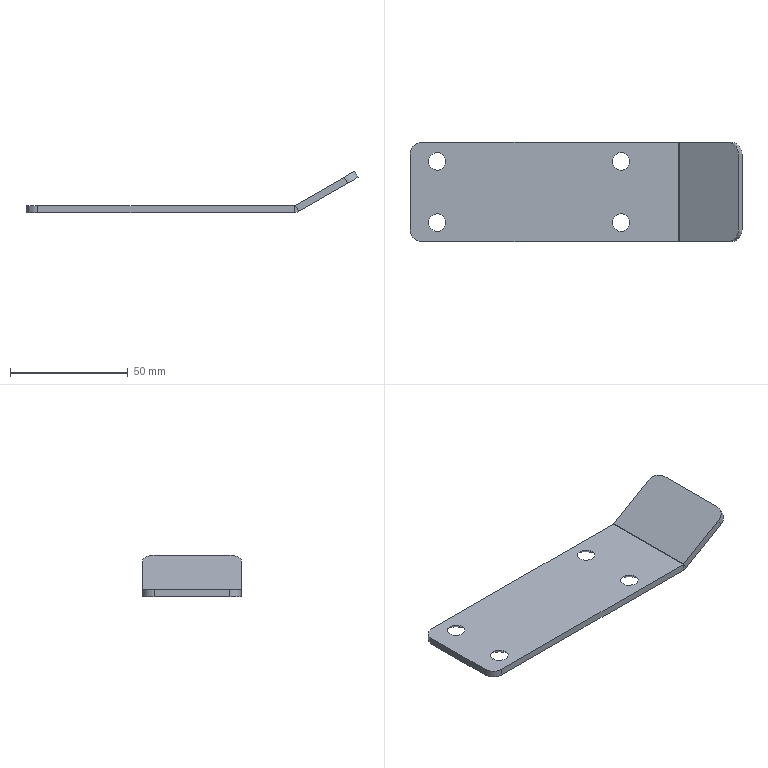Part | SolidWorks | features EdgeFlange 1, Fillet 1, FlatPattern 1, HoleWzd 1, SMBaseFlange 1, SheetMetal 1 | 1 solid | 26 faces | box 140.785 x 42 x 17.598 mm | volume 17021 mm3 | plane 12 | cone 8 | cylinder 6 | commonest cylinder face diameters 10 x4 1.473 x1 7.473 x1
STEP:
#1=CARTESIAN_POINT('',(-52.22,34.,0.));
#2=VERTEX_POINT('',#1);
#3=CARTESIAN_POINT('',(-44.78,34.,0.));
#4=VERTEX_POINT('',#3);
#5=CARTESIAN_POINT('',(-48.5,34.,0.));
#6=DIRECTION('',(0.,0.,1.));
#7=DIRECTION('',(1.,0.,0.));
#8=AXIS2_PLACEMENT_3D('',#5,#6,#7);
#9=CIRCLE('',#8,3.72);
#10=EDGE_CURVE('',#2,#4,#9,.T.);
#11=ORIENTED_EDGE('',*,*,#10,.T.);
#12=CARTESIAN_POINT('',(-41.78,34.,-3.));
#13=VERTEX_POINT('',#12);
#14=CARTESIAN_POINT('',(-41.78,34.,-3.));
#15=DIRECTION('',(0.7071,0.,-0.7071));
#16=VECTOR('',#15,1000.);
#17=LINE('',#14,#16);
#18=EDGE_CURVE('',#4,#13,#17,.T.);
#19=ORIENTED_EDGE('',*,*,#18,.T.);
#20=CARTESIAN_POINT('',(-55.22,34.,-3.));
#21=VERTEX_POINT('',#20);
#22=CARTESIAN_POINT('',(-48.5,34.,-3.));
#23=DIRECTION('',(0.,0.,-1.));
#24=DIRECTION('',(-1.,0.,0.));
#25=AXIS2_PLACEMENT_3D('',#22,#23,#24);
#26=CIRCLE('',#25,6.72);
#27=EDGE_CURVE('',#13,#21,#26,.T.);
#28=ORIENTED_EDGE('',*,*,#27,.T.);
#29=CARTESIAN_POINT('',(-55.22,34.,-3.));
#30=DIRECTION('',(-0.7071,0.,-0.7071));
#31=VECTOR('',#30,1000.);
#32=LINE('',#29,#31);
#33=EDGE_CURVE('',#2,#21,#32,.T.);
#34=ORIENTED_EDGE('',*,*,#33,.F.);
#35=EDGE_LOOP('',(#11,#19,#28,#34));
#36=FACE_OUTER_BOUND('',#35,.T.);
#37=CARTESIAN_POINT('',(-48.5,34.,-3.));
#38=DIRECTION('',(0.,0.,-1.));
#39=DIRECTION('',(-1.,0.,0.));
#40=AXIS2_PLACEMENT_3D('',#37,#38,#39);
#41=CONICAL_SURFACE('',#40,6.72,0.7854);
#42=ADVANCED_FACE('',(#36),#41,.F.);
#43=CARTESIAN_POINT('',(-52.22,8.,0.));
#44=VERTEX_POINT('',#43);
#45=CARTESIAN_POINT('',(-44.78,8.,0.));
#46=VERTEX_POINT('',#45);
#47=CARTESIAN_POINT('',(-48.5,8.,0.));
#48=DIRECTION('',(0.,0.,1.));
#49=DIRECTION('',(1.,0.,0.));
#50=AXIS2_PLACEMENT_3D('',#47,#48,#49);
#51=CIRCLE('',#50,3.72);
#52=EDGE_CURVE('',#44,#46,#51,.T.);
#53=ORIENTED_EDGE('',*,*,#52,.T.);
#54=CARTESIAN_POINT('',(-41.78,8.,-3.));
#55=VERTEX_POINT('',#54);
#56=CARTESIAN_POINT('',(-41.78,8.,-3.));
#57=DIRECTION('',(0.7071,0.,-0.7071));
#58=VECTOR('',#57,1000.);
#59=LINE('',#56,#58);
#60=EDGE_CURVE('',#46,#55,#59,.T.);
#61=ORIENTED_EDGE('',*,*,#60,.T.);
#62=CARTESIAN_POINT('',(-55.22,8.,-3.));
#63=VERTEX_POINT('',#62);
#64=CARTESIAN_POINT('',(-48.5,8.,-3.));
#65=DIRECTION('',(0.,0.,-1.));
#66=DIRECTION('',(-1.,0.,0.));
#67=AXIS2_PLACEMENT_3D('',#64,#65,#66);
#68=CIRCLE('',#67,6.72);
#69=EDGE_CURVE('',#55,#63,#68,.T.);
#70=ORIENTED_EDGE('',*,*,#69,.T.);
#71=CARTESIAN_POINT('',(-55.22,8.,-3.));
#72=DIRECTION('',(-0.7071,0.,-0.7071));
#73=VECTOR('',#72,1000.);
#74=LINE('',#71,#73);
#75=EDGE_CURVE('',#44,#63,#74,.T.);
#76=ORIENTED_EDGE('',*,*,#75,.F.);
#77=EDGE_LOOP('',(#53,#61,#70,#76));
#78=FACE_OUTER_BOUND('',#77,.T.);
#79=CARTESIAN_POINT('',(-48.5,8.,-3.));
#80=DIRECTION('',(0.,0.,-1.));
#81=DIRECTION('',(-1.,0.,0.));
#82=AXIS2_PLACEMENT_3D('',#79,#80,#81);
#83=CONICAL_SURFACE('',#82,6.72,0.7854);
#84=ADVANCED_FACE('',(#78),#83,.F.);
#85=CARTESIAN_POINT('',(25.78,34.,0.));
#86=VERTEX_POINT('',#85);
#87=CARTESIAN_POINT('',(33.22,34.,0.));
#88=VERTEX_POINT('',#87);
#89=CARTESIAN_POINT('',(29.5,34.,0.));
#90=DIRECTION('',(0.,0.,1.));
#91=DIRECTION('',(1.,0.,0.));
#92=AXIS2_PLACEMENT_3D('',#89,#90,#91);
#93=CIRCLE('',#92,3.72);
#94=EDGE_CURVE('',#86,#88,#93,.T.);
#95=ORIENTED_EDGE('',*,*,#94,.T.);
#96=CARTESIAN_POINT('',(36.22,34.,-3.));
#97=VERTEX_POINT('',#96);
#98=CARTESIAN_POINT('',(36.22,34.,-3.));
#99=DIRECTION('',(0.7071,0.,-0.7071));
#100=VECTOR('',#99,1000.);
#101=LINE('',#98,#100);
#102=EDGE_CURVE('',#88,#97,#101,.T.);
#103=ORIENTED_EDGE('',*,*,#102,.T.);
#104=CARTESIAN_POINT('',(22.78,34.,-3.));
#105=VERTEX_POINT('',#104);
#106=CARTESIAN_POINT('',(29.5,34.,-3.));
#107=DIRECTION('',(0.,0.,-1.));
#108=DIRECTION('',(-1.,0.,0.));
#109=AXIS2_PLACEMENT_3D('',#106,#107,#108);
#110=CIRCLE('',#109,6.72);
#111=EDGE_CURVE('',#97,#105,#110,.T.);
#112=ORIENTED_EDGE('',*,*,#111,.T.);
#113=CARTESIAN_POINT('',(22.78,34.,-3.));
#114=DIRECTION('',(-0.7071,0.,-0.7071));
#115=VECTOR('',#114,1000.);
#116=LINE('',#113,#115);
#117=EDGE_CURVE('',#86,#105,#116,.T.);
#118=ORIENTED_EDGE('',*,*,#117,.F.);
#119=EDGE_LOOP('',(#95,#103,#112,#118));
#120=FACE_OUTER_BOUND('',#119,.T.);
#121=CARTESIAN_POINT('',(29.5,34.,-3.));
#122=DIRECTION('',(0.,0.,-1.));
#123=DIRECTION('',(-1.,0.,0.));
#124=AXIS2_PLACEMENT_3D('',#121,#122,#123);
#125=CONICAL_SURFACE('',#124,6.72,0.7854);
#126=ADVANCED_FACE('',(#120),#125,.F.);
#127=CARTESIAN_POINT('',(25.78,8.,0.));
#128=VERTEX_POINT('',#127);
#129=CARTESIAN_POINT('',(33.22,8.,0.));
#130=VERTEX_POINT('',#129);
#131=CARTESIAN_POINT('',(29.5,8.,0.));
#132=DIRECTION('',(0.,0.,1.));
#133=DIRECTION('',(1.,0.,0.));
#134=AXIS2_PLACEMENT_3D('',#131,#132,#133);
#135=CIRCLE('',#134,3.72);
#136=EDGE_CURVE('',#128,#130,#135,.T.);
#137=ORIENTED_EDGE('',*,*,#136,.T.);
#138=CARTESIAN_POINT('',(36.22,8.,-3.));
#139=VERTEX_POINT('',#138);
#140=CARTESIAN_POINT('',(36.22,8.,-3.));
#141=DIRECTION('',(0.7071,0.,-0.7071));
#142=VECTOR('',#141,1000.);
#143=LINE('',#140,#142);
#144=EDGE_CURVE('',#130,#139,#143,.T.);
#145=ORIENTED_EDGE('',*,*,#144,.T.);
#146=CARTESIAN_POINT('',(22.78,8.,-3.));
#147=VERTEX_POINT('',#146);
#148=CARTESIAN_POINT('',(29.5,8.,-3.));
#149=DIRECTION('',(0.,0.,-1.));
#150=DIRECTION('',(-1.,0.,0.));
#151=AXIS2_PLACEMENT_3D('',#148,#149,#150);
#152=CIRCLE('',#151,6.72);
#153=EDGE_CURVE('',#139,#147,#152,.T.);
#154=ORIENTED_EDGE('',*,*,#153,.T.);
#155=CARTESIAN_POINT('',(22.78,8.,-3.));
#156=DIRECTION('',(-0.7071,0.,-0.7071));
#157=VECTOR('',#156,1000.);
#158=LINE('',#155,#157);
#159=EDGE_CURVE('',#128,#147,#158,.T.);
#160=ORIENTED_EDGE('',*,*,#159,.F.);
#161=EDGE_LOOP('',(#137,#145,#154,#160));
#162=FACE_OUTER_BOUND('',#161,.T.);
#163=CARTESIAN_POINT('',(29.5,8.,-3.));
#164=DIRECTION('',(0.,0.,-1.));
#165=DIRECTION('',(-1.,0.,0.));
#166=AXIS2_PLACEMENT_3D('',#163,#164,#165);
#167=CONICAL_SURFACE('',#166,6.72,0.7854);
#168=ADVANCED_FACE('',(#162),#167,.F.);
#169=CARTESIAN_POINT('',(53.803,42.,-3.));
#170=VERTEX_POINT('',#169);
#171=CARTESIAN_POINT('',(-55.,42.,-3.));
#172=VERTEX_POINT('',#171);
#173=CARTESIAN_POINT('',(-60.,42.,-3.));
#174=DIRECTION('',(-1.,0.,0.));
#175=VECTOR('',#174,1000.);
#176=LINE('',#173,#175);
#177=EDGE_CURVE('',#170,#172,#176,.T.);
#178=ORIENTED_EDGE('',*,*,#177,.T.);
#179=CARTESIAN_POINT('',(-55.,42.,0.));
#180=VERTEX_POINT('',#179);
#181=CARTESIAN_POINT('',(-55.,42.,-3.));
#182=DIRECTION('',(0.,0.,1.));
#183=VECTOR('',#182,1000.);
#184=LINE('',#181,#183);
#185=EDGE_CURVE('',#172,#180,#184,.T.);
#186=ORIENTED_EDGE('',*,*,#185,.T.);
#187=CARTESIAN_POINT('',(53.803,42.,0.));
#188=VERTEX_POINT('',#187);
#189=CARTESIAN_POINT('',(-60.,42.,0.));
#190=DIRECTION('',(-1.,0.,0.));
#191=VECTOR('',#190,1000.);
#192=LINE('',#189,#191);
#193=EDGE_CURVE('',#188,#180,#192,.T.);
#194=ORIENTED_EDGE('',*,*,#193,.F.);
#195=CARTESIAN_POINT('',(53.803,42.,0.));
#196=DIRECTION('',(0.,0.,-1.));
#197=VECTOR('',#196,1000.);
#198=LINE('',#195,#197);
#199=EDGE_CURVE('',#188,#170,#198,.T.);
#200=ORIENTED_EDGE('',*,*,#199,.T.);
#201=EDGE_LOOP('',(#178,#186,#194,#200));
#202=FACE_OUTER_BOUND('',#201,.T.);
#203=CARTESIAN_POINT('',(-60.,42.,-3.));
#204=DIRECTION('',(0.,1.,0.));
#205=DIRECTION('',(0.,0.,1.));
#206=AXIS2_PLACEMENT_3D('',#203,#204,#205);
#207=PLANE('',#206);
#208=ADVANCED_FACE('',(#202),#207,.T.);
#209=CARTESIAN_POINT('',(-48.5,34.,-3.));
#210=DIRECTION('',(0.,0.,-1.));
#211=DIRECTION('',(-1.,0.,0.));
#212=AXIS2_PLACEMENT_3D('',#209,#210,#211);
#213=CIRCLE('',#212,6.72);
#214=EDGE_CURVE('',#21,#13,#213,.T.);
#215=ORIENTED_EDGE('',*,*,#214,.F.);
#216=ORIENTED_EDGE('',*,*,#27,.F.);
#217=EDGE_LOOP('',(#215,#216));
#218=FACE_BOUND('',#217,.T.);
#219=CARTESIAN_POINT('',(-48.5,8.,-3.));
#220=DIRECTION('',(0.,0.,-1.));
#221=DIRECTION('',(-1.,0.,0.));
#222=AXIS2_PLACEMENT_3D('',#219,#220,#221);
#223=CIRCLE('',#222,6.72);
#224=EDGE_CURVE('',#63,#55,#223,.T.);
#225=ORIENTED_EDGE('',*,*,#224,.F.);
#226=ORIENTED_EDGE('',*,*,#69,.F.);
#227=EDGE_LOOP('',(#225,#226));
#228=FACE_BOUND('',#227,.T.);
#229=CARTESIAN_POINT('',(29.5,34.,-3.));
#230=DIRECTION('',(0.,0.,-1.));
#231=DIRECTION('',(-1.,0.,0.));
#232=AXIS2_PLACEMENT_3D('',#229,#230,#231);
#233=CIRCLE('',#232,6.72);
#234=EDGE_CURVE('',#105,#97,#233,.T.);
#235=ORIENTED_EDGE('',*,*,#234,.F.);
#236=ORIENTED_EDGE('',*,*,#111,.F.);
#237=EDGE_LOOP('',(#235,#236));
#238=FACE_BOUND('',#237,.T.);
#239=CARTESIAN_POINT('',(29.5,8.,-3.));
#240=DIRECTION('',(0.,0.,-1.));
#241=DIRECTION('',(-1.,0.,0.));
#242=AXIS2_PLACEMENT_3D('',#239,#240,#241);
#243=CIRCLE('',#242,6.72);
#244=EDGE_CURVE('',#147,#139,#243,.T.);
#245=ORIENTED_EDGE('',*,*,#244,.F.);
#246=ORIENTED_EDGE('',*,*,#153,.F.);
#247=EDGE_LOOP('',(#245,#246));
#248=FACE_BOUND('',#247,.T.);
#249=CARTESIAN_POINT('',(-55.,0.,-3.));
#250=VERTEX_POINT('',#249);
#251=CARTESIAN_POINT('',(53.803,0.,-3.));
#252=VERTEX_POINT('',#251);
#253=CARTESIAN_POINT('',(-60.,0.,-3.));
#254=DIRECTION('',(1.,0.,0.));
#255=VECTOR('',#254,1000.);
#256=LINE('',#253,#255);
#257=EDGE_CURVE('',#250,#252,#256,.T.);
#258=ORIENTED_EDGE('',*,*,#257,.F.);
#259=CARTESIAN_POINT('',(-60.,5.,-3.));
#260=VERTEX_POINT('',#259);
#261=CARTESIAN_POINT('',(-55.,5.,-3.));
#262=DIRECTION('',(0.,0.,-1.));
#263=DIRECTION('',(1.,0.,0.));
#264=AXIS2_PLACEMENT_3D('',#261,#262,#263);
#265=CIRCLE('',#264,5.);
#266=EDGE_CURVE('',#250,#260,#265,.T.);
#267=ORIENTED_EDGE('',*,*,#266,.T.);
#268=CARTESIAN_POINT('',(-60.,37.,-3.));
#269=VERTEX_POINT('',#268);
#270=CARTESIAN_POINT('',(-60.,42.,-3.));
#271=DIRECTION('',(0.,-1.,0.));
#272=VECTOR('',#271,1000.);
#273=LINE('',#270,#272);
#274=EDGE_CURVE('',#269,#260,#273,.T.);
#275=ORIENTED_EDGE('',*,*,#274,.F.);
#276=CARTESIAN_POINT('',(-55.,37.,-3.));
#277=DIRECTION('',(0.,0.,-1.));
#278=DIRECTION('',(1.,0.,0.));
#279=AXIS2_PLACEMENT_3D('',#276,#277,#278);
#280=CIRCLE('',#279,5.);
#281=EDGE_CURVE('',#269,#172,#280,.T.);
#282=ORIENTED_EDGE('',*,*,#281,.T.);
#283=ORIENTED_EDGE('',*,*,#177,.F.);
#284=CARTESIAN_POINT('',(53.803,42.,-3.));
#285=DIRECTION('',(0.,-1.,0.));
#286=VECTOR('',#285,1000.);
#287=LINE('',#284,#286);
#288=EDGE_CURVE('',#170,#252,#287,.T.);
#289=ORIENTED_EDGE('',*,*,#288,.T.);
#290=EDGE_LOOP('',(#258,#267,#275,#282,#283,#289));
#291=FACE_OUTER_BOUND('',#290,.T.);
#292=CARTESIAN_POINT('',(0.,0.,-3.));
#293=DIRECTION('',(0.,0.,1.));
#294=DIRECTION('',(1.,0.,0.));
#295=AXIS2_PLACEMENT_3D('',#292,#293,#294);
#296=PLANE('',#295);
#297=ADVANCED_FACE('',(#218,#228,#238,#248,#291),#296,.F.);
#298=ORIENTED_EDGE('',*,*,#10,.F.);
#299=CARTESIAN_POINT('',(-48.5,34.,0.));
#300=DIRECTION('',(0.,0.,1.));
#301=DIRECTION('',(1.,0.,0.));
#302=AXIS2_PLACEMENT_3D('',#299,#300,#301);
#303=CIRCLE('',#302,3.72);
#304=EDGE_CURVE('',#4,#2,#303,.T.);
#305=ORIENTED_EDGE('',*,*,#304,.F.);
#306=EDGE_LOOP('',(#298,#305));
#307=FACE_BOUND('',#306,.T.);
#308=ORIENTED_EDGE('',*,*,#52,.F.);
#309=CARTESIAN_POINT('',(-48.5,8.,0.));
#310=DIRECTION('',(0.,0.,1.));
#311=DIRECTION('',(1.,0.,0.));
#312=AXIS2_PLACEMENT_3D('',#309,#310,#311);
#313=CIRCLE('',#312,3.72);
#314=EDGE_CURVE('',#46,#44,#313,.T.);
#315=ORIENTED_EDGE('',*,*,#314,.F.);
#316=EDGE_LOOP('',(#308,#315));
#317=FACE_BOUND('',#316,.T.);
#318=ORIENTED_EDGE('',*,*,#94,.F.);
#319=CARTESIAN_POINT('',(29.5,34.,0.));
#320=DIRECTION('',(0.,0.,1.));
#321=DIRECTION('',(1.,0.,0.));
#322=AXIS2_PLACEMENT_3D('',#319,#320,#321);
#323=CIRCLE('',#322,3.72);
#324=EDGE_CURVE('',#88,#86,#323,.T.);
#325=ORIENTED_EDGE('',*,*,#324,.F.);
#326=EDGE_LOOP('',(#318,#325));
#327=FACE_BOUND('',#326,.T.);
#328=ORIENTED_EDGE('',*,*,#136,.F.);
#329=CARTESIAN_POINT('',(29.5,8.,0.));
#330=DIRECTION('',(0.,0.,1.));
#331=DIRECTION('',(1.,0.,0.));
#332=AXIS2_PLACEMENT_3D('',#329,#330,#331);
#333=CIRCLE('',#332,3.72);
#334=EDGE_CURVE('',#130,#128,#333,.T.);
#335=ORIENTED_EDGE('',*,*,#334,.F.);
#336=EDGE_LOOP('',(#328,#335));
#337=FACE_BOUND('',#336,.T.);
#338=CARTESIAN_POINT('',(-60.,37.,0.));
#339=VERTEX_POINT('',#338);
#340=CARTESIAN_POINT('',(-60.,5.,0.));
#341=VERTEX_POINT('',#340);
#342=CARTESIAN_POINT('',(-60.,42.,0.));
#343=DIRECTION('',(0.,-1.,0.));
#344=VECTOR('',#343,1000.);
#345=LINE('',#342,#344);
#346=EDGE_CURVE('',#339,#341,#345,.T.);
#347=ORIENTED_EDGE('',*,*,#346,.T.);
#348=CARTESIAN_POINT('',(-55.,0.,0.));
#349=VERTEX_POINT('',#348);
#350=CARTESIAN_POINT('',(-55.,5.,0.));
#351=DIRECTION('',(0.,0.,1.));
#352=DIRECTION('',(1.,0.,0.));
#353=AXIS2_PLACEMENT_3D('',#350,#351,#352);
#354=CIRCLE('',#353,5.);
#355=EDGE_CURVE('',#341,#349,#354,.T.);
#356=ORIENTED_EDGE('',*,*,#355,.T.);
#357=CARTESIAN_POINT('',(53.803,0.,0.));
#358=VERTEX_POINT('',#357);
#359=CARTESIAN_POINT('',(-60.,0.,0.));
#360=DIRECTION('',(1.,0.,0.));
#361=VECTOR('',#360,1000.);
#362=LINE('',#359,#361);
#363=EDGE_CURVE('',#349,#358,#362,.T.);
#364=ORIENTED_EDGE('',*,*,#363,.T.);
#365=CARTESIAN_POINT('',(53.803,42.,0.));
#366=DIRECTION('',(0.,-1.,0.));
#367=VECTOR('',#366,1000.);
#368=LINE('',#365,#367);
#369=EDGE_CURVE('',#188,#358,#368,.T.);
#370=ORIENTED_EDGE('',*,*,#369,.F.);
#371=ORIENTED_EDGE('',*,*,#193,.T.);
#372=CARTESIAN_POINT('',(-55.,37.,0.));
#373=DIRECTION('',(0.,0.,1.));
#374=DIRECTION('',(1.,0.,0.));
#375=AXIS2_PLACEMENT_3D('',#372,#373,#374);
#376=CIRCLE('',#375,5.);
#377=EDGE_CURVE('',#180,#339,#376,.T.);
#378=ORIENTED_EDGE('',*,*,#377,.T.);
#379=EDGE_LOOP('',(#347,#356,#364,#370,#371,#378));
#380=FACE_OUTER_BOUND('',#379,.T.);
#381=CARTESIAN_POINT('',(0.,0.,0.));
#382=DIRECTION('',(0.,0.,1.));
#383=DIRECTION('',(1.,0.,0.));
#384=AXIS2_PLACEMENT_3D('',#381,#382,#383);
#385=PLANE('',#384);
#386=ADVANCED_FACE('',(#307,#317,#327,#337,#380),#385,.T.);
#387=ORIENTED_EDGE('',*,*,#274,.T.);
#388=CARTESIAN_POINT('',(-60.,5.,-3.));
#389=DIRECTION('',(0.,0.,1.));
#390=VECTOR('',#389,1000.);
#391=LINE('',#388,#390);
#392=EDGE_CURVE('',#260,#341,#391,.T.);
#393=ORIENTED_EDGE('',*,*,#392,.T.);
#394=ORIENTED_EDGE('',*,*,#346,.F.);
#395=CARTESIAN_POINT('',(-60.,37.,-3.));
#396=DIRECTION('',(0.,0.,-1.));
#397=VECTOR('',#396,1000.);
#398=LINE('',#395,#397);
#399=EDGE_CURVE('',#339,#269,#398,.T.);
#400=ORIENTED_EDGE('',*,*,#399,.T.);
#401=EDGE_LOOP('',(#387,#393,#394,#400));
#402=FACE_OUTER_BOUND('',#401,.T.);
#403=CARTESIAN_POINT('',(-60.,42.,-3.));
#404=DIRECTION('',(-1.,0.,0.));
#405=DIRECTION('',(0.,0.,1.));
#406=AXIS2_PLACEMENT_3D('',#403,#404,#405);
#407=PLANE('',#406);
#408=ADVANCED_FACE('',(#402),#407,.T.);
#409=ORIENTED_EDGE('',*,*,#363,.F.);
#410=CARTESIAN_POINT('',(-55.,0.,-3.));
#411=DIRECTION('',(0.,0.,-1.));
#412=VECTOR('',#411,1000.);
#413=LINE('',#410,#412);
#414=EDGE_CURVE('',#349,#250,#413,.T.);
#415=ORIENTED_EDGE('',*,*,#414,.T.);
#416=ORIENTED_EDGE('',*,*,#257,.T.);
#417=CARTESIAN_POINT('',(53.803,0.,0.));
#418=DIRECTION('',(0.,0.,-1.));
#419=VECTOR('',#418,1000.);
#420=LINE('',#417,#419);
#421=EDGE_CURVE('',#358,#252,#420,.T.);
#422=ORIENTED_EDGE('',*,*,#421,.F.);
#423=EDGE_LOOP('',(#409,#415,#416,#422));
#424=FACE_OUTER_BOUND('',#423,.T.);
#425=CARTESIAN_POINT('',(-60.,0.,-3.));
#426=DIRECTION('',(0.,-1.,0.));
#427=DIRECTION('',(0.,0.,-1.));
#428=AXIS2_PLACEMENT_3D('',#425,#426,#427);
#429=PLANE('',#428);
#430=ADVANCED_FACE('',(#424),#429,.T.);
#431=CARTESIAN_POINT('',(54.171,0.,0.09869));
#432=VERTEX_POINT('',#431);
#433=CARTESIAN_POINT('',(55.671,0.,-2.499));
#434=VERTEX_POINT('',#433);
#435=CARTESIAN_POINT('',(55.671,0.,-2.499));
#436=DIRECTION('',(0.5,0.,-0.866));
#437=VECTOR('',#436,1000.);
#438=LINE('',#435,#437);
#439=EDGE_CURVE('',#432,#434,#438,.T.);
#440=ORIENTED_EDGE('',*,*,#439,.F.);
#441=CARTESIAN_POINT('',(53.803,0.,0.7366));
#442=DIRECTION('',(0.,-1.,0.));
#443=DIRECTION('',(0.,0.,1.));
#444=AXIS2_PLACEMENT_3D('',#441,#442,#443);
#445=CIRCLE('',#444,0.7366);
#446=EDGE_CURVE('',#358,#432,#445,.T.);
#447=ORIENTED_EDGE('',*,*,#446,.F.);
#448=ORIENTED_EDGE('',*,*,#421,.T.);
#449=CARTESIAN_POINT('',(53.803,0.,0.7366));
#450=DIRECTION('',(0.,-1.,0.));
#451=DIRECTION('',(0.,0.,1.));
#452=AXIS2_PLACEMENT_3D('',#449,#450,#451);
#453=CIRCLE('',#452,3.737);
#454=EDGE_CURVE('',#252,#434,#453,.T.);
#455=ORIENTED_EDGE('',*,*,#454,.T.);
#456=EDGE_LOOP('',(#440,#447,#448,#455));
#457=FACE_OUTER_BOUND('',#456,.T.);
#458=CARTESIAN_POINT('',(53.803,0.,0.7366));
#459=DIRECTION('',(0.,-1.,0.));
#460=DIRECTION('',(0.,0.,-1.));
#461=AXIS2_PLACEMENT_3D('',#458,#459,#460);
#462=PLANE('',#461);
#463=ADVANCED_FACE('',(#457),#462,.T.);
#464=CARTESIAN_POINT('',(54.171,42.,0.09869));
#465=VERTEX_POINT('',#464);
#466=CARTESIAN_POINT('',(53.803,42.,0.7366));
#467=DIRECTION('',(0.,1.,0.));
#468=DIRECTION('',(0.,0.,1.));
#469=AXIS2_PLACEMENT_3D('',#466,#467,#468);
#470=CIRCLE('',#469,0.7366);
#471=EDGE_CURVE('',#465,#188,#470,.T.);
#472=ORIENTED_EDGE('',*,*,#471,.F.);
#473=CARTESIAN_POINT('',(55.671,42.,-2.499));
#474=VERTEX_POINT('',#473);
#475=CARTESIAN_POINT('',(54.171,42.,0.09869));
#476=DIRECTION('',(0.5,0.,-0.866));
#477=VECTOR('',#476,1000.);
#478=LINE('',#475,#477);
#479=EDGE_CURVE('',#465,#474,#478,.T.);
#480=ORIENTED_EDGE('',*,*,#479,.T.);
#481=CARTESIAN_POINT('',(53.803,42.,0.7366));
#482=DIRECTION('',(0.,1.,0.));
#483=DIRECTION('',(0.,0.,1.));
#484=AXIS2_PLACEMENT_3D('',#481,#482,#483);
#485=CIRCLE('',#484,3.737);
#486=EDGE_CURVE('',#474,#170,#485,.T.);
#487=ORIENTED_EDGE('',*,*,#486,.T.);
#488=ORIENTED_EDGE('',*,*,#199,.F.);
#489=EDGE_LOOP('',(#472,#480,#487,#488));
#490=FACE_OUTER_BOUND('',#489,.T.);
#491=CARTESIAN_POINT('',(53.803,42.,0.7366));
#492=DIRECTION('',(0.,-1.,0.));
#493=DIRECTION('',(0.,0.,-1.));
#494=AXIS2_PLACEMENT_3D('',#491,#492,#493);
#495=PLANE('',#494);
#496=ADVANCED_FACE('',(#490),#495,.F.);
#497=ORIENTED_EDGE('',*,*,#288,.F.);
#498=ORIENTED_EDGE('',*,*,#486,.F.);
#499=CARTESIAN_POINT('',(55.671,0.,-2.499));
#500=DIRECTION('',(0.,-1.,0.));
#501=VECTOR('',#500,1000.);
#502=LINE('',#499,#501);
#503=EDGE_CURVE('',#474,#434,#502,.T.);
#504=ORIENTED_EDGE('',*,*,#503,.T.);
#505=ORIENTED_EDGE('',*,*,#454,.F.);
#506=EDGE_LOOP('',(#497,#498,#504,#505));
#507=FACE_OUTER_BOUND('',#506,.T.);
#508=CARTESIAN_POINT('',(53.803,42.,0.7366));
#509=DIRECTION('',(0.,1.,0.));
#510=DIRECTION('',(0.5,0.,-0.866));
#511=AXIS2_PLACEMENT_3D('',#508,#509,#510);
#512=CYLINDRICAL_SURFACE('',#511,3.737);
#513=ADVANCED_FACE('',(#507),#512,.T.);
#514=ORIENTED_EDGE('',*,*,#369,.T.);
#515=ORIENTED_EDGE('',*,*,#446,.T.);
#516=CARTESIAN_POINT('',(54.171,0.,0.09869));
#517=DIRECTION('',(0.,1.,0.));
#518=VECTOR('',#517,1000.);
#519=LINE('',#516,#518);
#520=EDGE_CURVE('',#432,#465,#519,.T.);
#521=ORIENTED_EDGE('',*,*,#520,.T.);
#522=ORIENTED_EDGE('',*,*,#471,.T.);
#523=EDGE_LOOP('',(#514,#515,#521,#522));
#524=FACE_OUTER_BOUND('',#523,.T.);
#525=CARTESIAN_POINT('',(53.803,42.,0.7366));
#526=DIRECTION('',(0.,1.,0.));
#527=DIRECTION('',(0.5,0.,-0.866));
#528=AXIS2_PLACEMENT_3D('',#525,#526,#527);
#529=CYLINDRICAL_SURFACE('',#528,0.7366);
#530=ADVANCED_FACE('',(#524),#529,.F.);
#531=CARTESIAN_POINT('',(76.454,0.,9.5));
#532=VERTEX_POINT('',#531);
#533=CARTESIAN_POINT('',(10.5,0.,-28.579));
#534=DIRECTION('',(-0.866,0.,-0.5));
#535=VECTOR('',#534,1000.);
#536=LINE('',#533,#535);
#537=EDGE_CURVE('',#532,#434,#536,.T.);
#538=ORIENTED_EDGE('',*,*,#537,.F.);
#539=CARTESIAN_POINT('',(74.954,0.,12.098));
#540=VERTEX_POINT('',#539);
#541=CARTESIAN_POINT('',(76.454,0.,9.5));
#542=DIRECTION('',(-0.5,0.,0.866));
#543=VECTOR('',#542,1000.);
#544=LINE('',#541,#543);
#545=EDGE_CURVE('',#532,#540,#544,.T.);
#546=ORIENTED_EDGE('',*,*,#545,.T.);
#547=CARTESIAN_POINT('',(54.,0.,0.));
#548=DIRECTION('',(-0.866,0.,-0.5));
#549=VECTOR('',#548,1000.);
#550=LINE('',#547,#549);
#551=EDGE_CURVE('',#540,#432,#550,.T.);
#552=ORIENTED_EDGE('',*,*,#551,.T.);
#553=ORIENTED_EDGE('',*,*,#439,.T.);
#554=EDGE_LOOP('',(#538,#546,#552,#553));
#555=FACE_OUTER_BOUND('',#554,.T.);
#556=CARTESIAN_POINT('',(55.5,0.,-2.598));
#557=DIRECTION('',(0.,1.,0.));
#558=DIRECTION('',(0.,0.,1.));
#559=AXIS2_PLACEMENT_3D('',#556,#557,#558);
#560=PLANE('',#559);
#561=ADVANCED_FACE('',(#555),#560,.F.);
#562=CARTESIAN_POINT('',(74.954,42.,12.098));
#563=VERTEX_POINT('',#562);
#564=CARTESIAN_POINT('',(79.285,42.,14.598));
#565=DIRECTION('',(0.866,0.,0.5));
#566=VECTOR('',#565,1000.);
#567=LINE('',#564,#566);
#568=EDGE_CURVE('',#465,#563,#567,.T.);
#569=ORIENTED_EDGE('',*,*,#568,.T.);
#570=CARTESIAN_POINT('',(76.454,42.,9.5));
#571=VERTEX_POINT('',#570);
#572=CARTESIAN_POINT('',(76.454,42.,9.5));
#573=DIRECTION('',(0.5,0.,-0.866));
#574=VECTOR('',#573,1000.);
#575=LINE('',#572,#574);
#576=EDGE_CURVE('',#563,#571,#575,.T.);
#577=ORIENTED_EDGE('',*,*,#576,.T.);
#578=CARTESIAN_POINT('',(10.5,42.,-28.579));
#579=DIRECTION('',(0.866,0.,0.5));
#580=VECTOR('',#579,1000.);
#581=LINE('',#578,#580);
#582=EDGE_CURVE('',#474,#571,#581,.T.);
#583=ORIENTED_EDGE('',*,*,#582,.F.);
#584=ORIENTED_EDGE('',*,*,#479,.F.);
#585=EDGE_LOOP('',(#569,#577,#583,#584));
#586=FACE_OUTER_BOUND('',#585,.T.);
#587=CARTESIAN_POINT('',(80.785,42.,12.));
#588=DIRECTION('',(0.,-1.,0.));
#589=DIRECTION('',(1.,0.,0.));
#590=AXIS2_PLACEMENT_3D('',#587,#588,#589);
#591=PLANE('',#590);
#592=ADVANCED_FACE('',(#586),#591,.F.);
#593=CARTESIAN_POINT('',(80.785,37.,12.));
#594=VERTEX_POINT('',#593);
#595=CARTESIAN_POINT('',(80.785,5.,12.));
#596=VERTEX_POINT('',#595);
#597=CARTESIAN_POINT('',(80.785,0.,12.));
#598=DIRECTION('',(0.,-1.,0.));
#599=VECTOR('',#598,1000.);
#600=LINE('',#597,#599);
#601=EDGE_CURVE('',#594,#596,#600,.T.);
#602=ORIENTED_EDGE('',*,*,#601,.T.);
#603=CARTESIAN_POINT('',(76.454,5.,9.5));
#604=DIRECTION('',(0.5,0.,-0.866));
#605=DIRECTION('',(0.866,0.,0.5));
#606=AXIS2_PLACEMENT_3D('',#603,#604,#605);
#607=CIRCLE('',#606,5.);
#608=EDGE_CURVE('',#596,#532,#607,.T.);
#609=ORIENTED_EDGE('',*,*,#608,.T.);
#610=ORIENTED_EDGE('',*,*,#537,.T.);
#611=ORIENTED_EDGE('',*,*,#503,.F.);
#612=ORIENTED_EDGE('',*,*,#582,.T.);
#613=CARTESIAN_POINT('',(76.454,37.,9.5));
#614=DIRECTION('',(0.5,0.,-0.866));
#615=DIRECTION('',(0.866,0.,0.5));
#616=AXIS2_PLACEMENT_3D('',#613,#614,#615);
#617=CIRCLE('',#616,5.);
#618=EDGE_CURVE('',#571,#594,#617,.T.);
#619=ORIENTED_EDGE('',*,*,#618,.T.);
#620=EDGE_LOOP('',(#602,#609,#610,#611,#612,#619));
#621=FACE_OUTER_BOUND('',#620,.T.);
#622=CARTESIAN_POINT('',(10.5,0.,-28.579));
#623=DIRECTION('',(-0.5,0.,0.866));
#624=DIRECTION('',(0.866,0.,0.5));
#625=AXIS2_PLACEMENT_3D('',#622,#623,#624);
#626=PLANE('',#625);
#627=ADVANCED_FACE('',(#621),#626,.F.);
#628=ORIENTED_EDGE('',*,*,#551,.F.);
#629=CARTESIAN_POINT('',(79.285,5.,14.598));
#630=VERTEX_POINT('',#629);
#631=CARTESIAN_POINT('',(74.954,5.,12.098));
#632=DIRECTION('',(-0.5,0.,0.866));
#633=DIRECTION('',(0.866,0.,0.5));
#634=AXIS2_PLACEMENT_3D('',#631,#632,#633);
#635=CIRCLE('',#634,5.);
#636=EDGE_CURVE('',#540,#630,#635,.T.);
#637=ORIENTED_EDGE('',*,*,#636,.T.);
#638=CARTESIAN_POINT('',(79.285,37.,14.598));
#639=VERTEX_POINT('',#638);
#640=CARTESIAN_POINT('',(79.285,0.,14.598));
#641=DIRECTION('',(0.,-1.,0.));
#642=VECTOR('',#641,1000.);
#643=LINE('',#640,#642);
#644=EDGE_CURVE('',#639,#630,#643,.T.);
#645=ORIENTED_EDGE('',*,*,#644,.F.);
#646=CARTESIAN_POINT('',(74.954,37.,12.098));
#647=DIRECTION('',(-0.5,0.,0.866));
#648=DIRECTION('',(0.866,0.,0.5));
#649=AXIS2_PLACEMENT_3D('',#646,#647,#648);
#650=CIRCLE('',#649,5.);
#651=EDGE_CURVE('',#639,#563,#650,.T.);
#652=ORIENTED_EDGE('',*,*,#651,.T.);
#653=ORIENTED_EDGE('',*,*,#568,.F.);
#654=ORIENTED_EDGE('',*,*,#520,.F.);
#655=EDGE_LOOP('',(#628,#637,#645,#652,#653,#654));
#656=FACE_OUTER_BOUND('',#655,.T.);
#657=CARTESIAN_POINT('',(9.,0.,-25.981));
#658=DIRECTION('',(-0.5,0.,0.866));
#659=DIRECTION('',(0.866,0.,0.5));
#660=AXIS2_PLACEMENT_3D('',#657,#658,#659);
#661=PLANE('',#660);
#662=ADVANCED_FACE('',(#656),#661,.T.);
#663=ORIENTED_EDGE('',*,*,#644,.T.);
#664=CARTESIAN_POINT('',(80.785,5.,12.));
#665=DIRECTION('',(0.5,0.,-0.866));
#666=VECTOR('',#665,1000.);
#667=LINE('',#664,#666);
#668=EDGE_CURVE('',#630,#596,#667,.T.);
#669=ORIENTED_EDGE('',*,*,#668,.T.);
#670=ORIENTED_EDGE('',*,*,#601,.F.);
#671=CARTESIAN_POINT('',(80.785,37.,12.));
#672=DIRECTION('',(-0.5,0.,0.866));
#673=VECTOR('',#672,1000.);
#674=LINE('',#671,#673);
#675=EDGE_CURVE('',#594,#639,#674,.T.);
#676=ORIENTED_EDGE('',*,*,#675,.T.);
#677=EDGE_LOOP('',(#663,#669,#670,#676));
#678=FACE_OUTER_BOUND('',#677,.T.);
#679=CARTESIAN_POINT('',(80.785,0.,12.));
#680=DIRECTION('',(-0.866,0.,-0.5));
#681=DIRECTION('',(-0.5,0.,0.866));
#682=AXIS2_PLACEMENT_3D('',#679,#680,#681);
#683=PLANE('',#682);
#684=ADVANCED_FACE('',(#678),#683,.F.);
#685=ORIENTED_EDGE('',*,*,#266,.F.);
#686=ORIENTED_EDGE('',*,*,#414,.F.);
#687=ORIENTED_EDGE('',*,*,#355,.F.);
#688=ORIENTED_EDGE('',*,*,#392,.F.);
#689=EDGE_LOOP('',(#685,#686,#687,#688));
#690=FACE_OUTER_BOUND('',#689,.T.);
#691=CARTESIAN_POINT('',(-55.,5.,-3.));
#692=DIRECTION('',(0.,0.,1.));
#693=DIRECTION('',(1.,0.,0.));
#694=AXIS2_PLACEMENT_3D('',#691,#692,#693);
#695=CYLINDRICAL_SURFACE('',#694,5.);
#696=ADVANCED_FACE('',(#690),#695,.T.);
#697=ORIENTED_EDGE('',*,*,#281,.F.);
#698=ORIENTED_EDGE('',*,*,#399,.F.);
#699=ORIENTED_EDGE('',*,*,#377,.F.);
#700=ORIENTED_EDGE('',*,*,#185,.F.);
#701=EDGE_LOOP('',(#697,#698,#699,#700));
#702=FACE_OUTER_BOUND('',#701,.T.);
#703=CARTESIAN_POINT('',(-55.,37.,-3.));
#704=DIRECTION('',(0.,0.,1.));
#705=DIRECTION('',(1.,0.,0.));
#706=AXIS2_PLACEMENT_3D('',#703,#704,#705);
#707=CYLINDRICAL_SURFACE('',#706,5.);
#708=ADVANCED_FACE('',(#702),#707,.T.);
#709=ORIENTED_EDGE('',*,*,#608,.F.);
#710=ORIENTED_EDGE('',*,*,#668,.F.);
#711=ORIENTED_EDGE('',*,*,#636,.F.);
#712=ORIENTED_EDGE('',*,*,#545,.F.);
#713=EDGE_LOOP('',(#709,#710,#711,#712));
#714=FACE_OUTER_BOUND('',#713,.T.);
#715=CARTESIAN_POINT('',(76.454,5.,9.5));
#716=DIRECTION('',(-0.5,0.,0.866));
#717=DIRECTION('',(0.866,0.,0.5));
#718=AXIS2_PLACEMENT_3D('',#715,#716,#717);
#719=CYLINDRICAL_SURFACE('',#718,5.);
#720=ADVANCED_FACE('',(#714),#719,.T.);
#721=ORIENTED_EDGE('',*,*,#618,.F.);
#722=ORIENTED_EDGE('',*,*,#576,.F.);
#723=ORIENTED_EDGE('',*,*,#651,.F.);
#724=ORIENTED_EDGE('',*,*,#675,.F.);
#725=EDGE_LOOP('',(#721,#722,#723,#724));
#726=FACE_OUTER_BOUND('',#725,.T.);
#727=CARTESIAN_POINT('',(76.454,37.,9.5));
#728=DIRECTION('',(-0.5,0.,0.866));
#729=DIRECTION('',(0.866,0.,0.5));
#730=AXIS2_PLACEMENT_3D('',#727,#728,#729);
#731=CYLINDRICAL_SURFACE('',#730,5.);
#732=ADVANCED_FACE('',(#726),#731,.T.);
#733=ORIENTED_EDGE('',*,*,#144,.F.);
#734=ORIENTED_EDGE('',*,*,#334,.T.);
#735=ORIENTED_EDGE('',*,*,#159,.T.);
#736=ORIENTED_EDGE('',*,*,#244,.T.);
#737=EDGE_LOOP('',(#733,#734,#735,#736));
#738=FACE_OUTER_BOUND('',#737,.T.);
#739=CARTESIAN_POINT('',(29.5,8.,-3.));
#740=DIRECTION('',(0.,0.,-1.));
#741=DIRECTION('',(-1.,0.,0.));
#742=AXIS2_PLACEMENT_3D('',#739,#740,#741);
#743=CONICAL_SURFACE('',#742,6.72,0.7854);
#744=ADVANCED_FACE('',(#738),#743,.F.);
#745=ORIENTED_EDGE('',*,*,#102,.F.);
#746=ORIENTED_EDGE('',*,*,#324,.T.);
#747=ORIENTED_EDGE('',*,*,#117,.T.);
#748=ORIENTED_EDGE('',*,*,#234,.T.);
#749=EDGE_LOOP('',(#745,#746,#747,#748));
#750=FACE_OUTER_BOUND('',#749,.T.);
#751=CARTESIAN_POINT('',(29.5,34.,-3.));
#752=DIRECTION('',(0.,0.,-1.));
#753=DIRECTION('',(-1.,0.,0.));
#754=AXIS2_PLACEMENT_3D('',#751,#752,#753);
#755=CONICAL_SURFACE('',#754,6.72,0.7854);
#756=ADVANCED_FACE('',(#750),#755,.F.);
#757=ORIENTED_EDGE('',*,*,#60,.F.);
#758=ORIENTED_EDGE('',*,*,#314,.T.);
#759=ORIENTED_EDGE('',*,*,#75,.T.);
#760=ORIENTED_EDGE('',*,*,#224,.T.);
#761=EDGE_LOOP('',(#757,#758,#759,#760));
#762=FACE_OUTER_BOUND('',#761,.T.);
#763=CARTESIAN_POINT('',(-48.5,8.,-3.));
#764=DIRECTION('',(0.,0.,-1.));
#765=DIRECTION('',(-1.,0.,0.));
#766=AXIS2_PLACEMENT_3D('',#763,#764,#765);
#767=CONICAL_SURFACE('',#766,6.72,0.7854);
#768=ADVANCED_FACE('',(#762),#767,.F.);
#769=ORIENTED_EDGE('',*,*,#18,.F.);
#770=ORIENTED_EDGE('',*,*,#304,.T.);
#771=ORIENTED_EDGE('',*,*,#33,.T.);
#772=ORIENTED_EDGE('',*,*,#214,.T.);
#773=EDGE_LOOP('',(#769,#770,#771,#772));
#774=FACE_OUTER_BOUND('',#773,.T.);
#775=CARTESIAN_POINT('',(-48.5,34.,-3.));
#776=DIRECTION('',(0.,0.,-1.));
#777=DIRECTION('',(-1.,0.,0.));
#778=AXIS2_PLACEMENT_3D('',#775,#776,#777);
#779=CONICAL_SURFACE('',#778,6.72,0.7854);
#780=ADVANCED_FACE('',(#774),#779,.F.);
#781=CLOSED_SHELL('',(#42,#84,#126,#168,#208,#297,#386,#408,#430,#463,#496,#513,#530,#561,#592,#627,#662,#684,#696,#708,#720,#732,#744,#756,#768,#780));
#782=MANIFOLD_SOLID_BREP('',#781);
#783=CARTESIAN_POINT('',(0.,0.,0.));
#784=DIRECTION('',(0.,0.,1.));
#785=DIRECTION('',(1.,0.,0.));
#786=AXIS2_PLACEMENT_3D('',#783,#784,#785);
#787=(LENGTH_UNIT()NAMED_UNIT(*)SI_UNIT(.MILLI.,.METRE.));
#788=UNCERTAINTY_MEASURE_WITH_UNIT(LENGTH_MEASURE(0.00001),#787,'','');
#789=(NAMED_UNIT(*)PLANE_ANGLE_UNIT()SI_UNIT($,.RADIAN.));
#790=(NAMED_UNIT(*)SI_UNIT($,.STERADIAN.)SOLID_ANGLE_UNIT());
#791=(GEOMETRIC_REPRESENTATION_CONTEXT(3)GLOBAL_UNCERTAINTY_ASSIGNED_CONTEXT((#788))GLOBAL_UNIT_ASSIGNED_CONTEXT((#787,#789,#790))REPRESENTATION_CONTEXT('',''));
#792=ADVANCED_BREP_SHAPE_REPRESENTATION('',(#782,#786),#791);